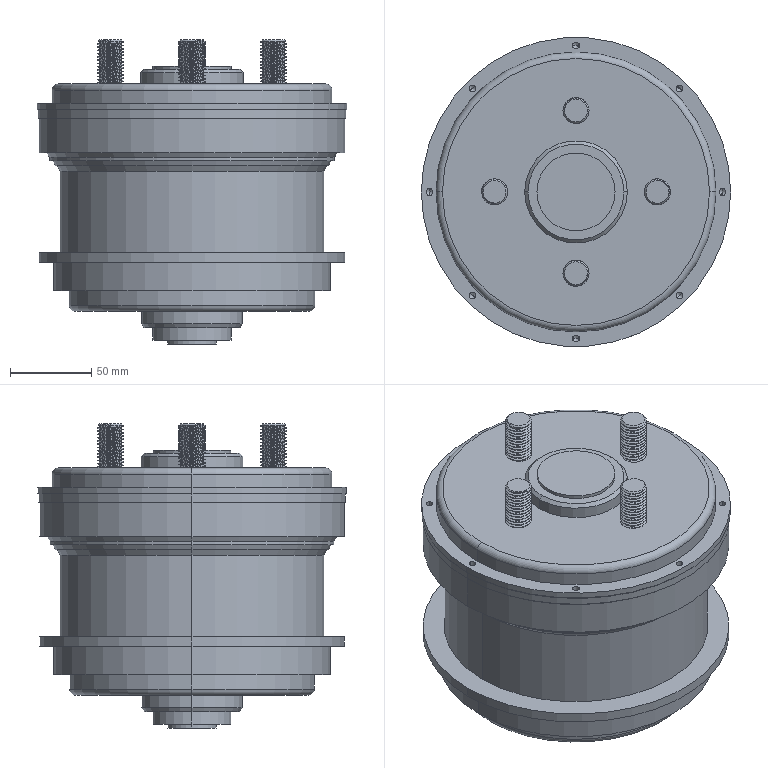Part | SolidWorks | features CirPattern 2, HoleWzd 2, ICE 2, Chamfer 1, Revolution 1, SweepThread 1 | 5 solids | 266 faces | box 190 x 190 x 186.81 mm | volume 3283817 mm3 | cylinder 170 | cone 52 | plane 28 | spline 12 | torus 4 | commonest cylinder face diameters 16 x108 4.2 x32 48 x4 188 x4 20 x2 30 x2